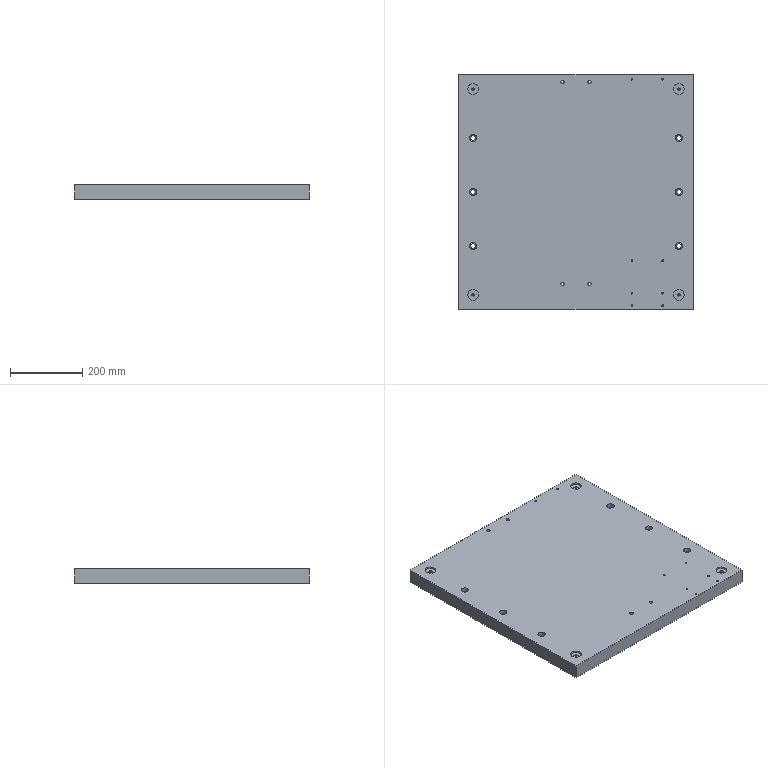Part | SolidWorks | features BaseBody 1 | 1 solid | 112 faces | box 650 x 650 x 40 mm | volume 16789286 mm3 | cylinder 80 | plane 24 | cone 8 | commonest cylinder face diameters 13.5 x20 20 x20 5 x16 9 x8 15 x8 30 x8